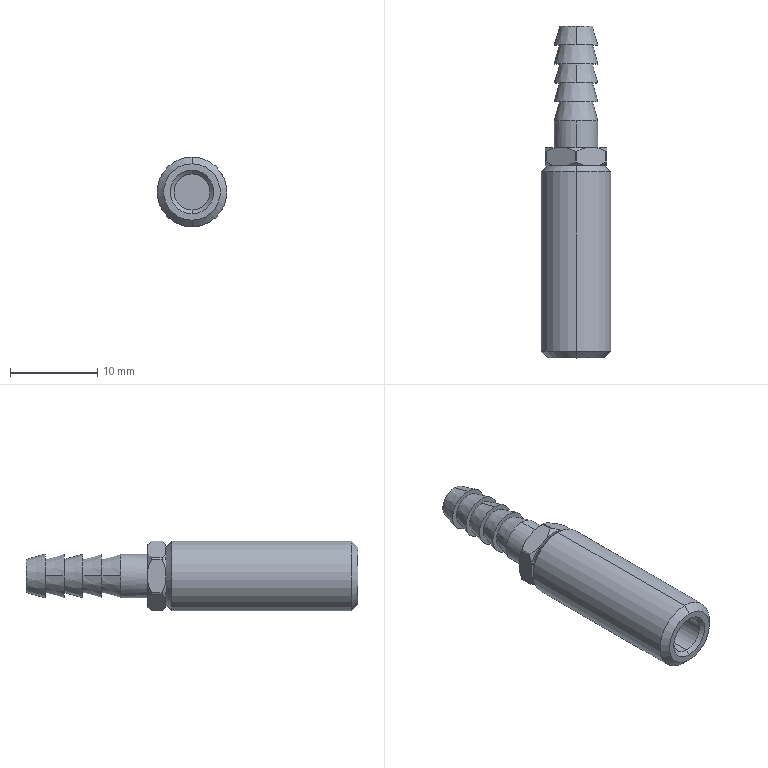Part | SolidWorks | features BaseBody 1 | 1 solid | 57 faces | box 8 x 38 x 8 mm | volume 1345 mm3 | cone 29 | plane 15 | cylinder 13 | commonest cylinder face diameters 8 x9 4.134 x2 5 x2